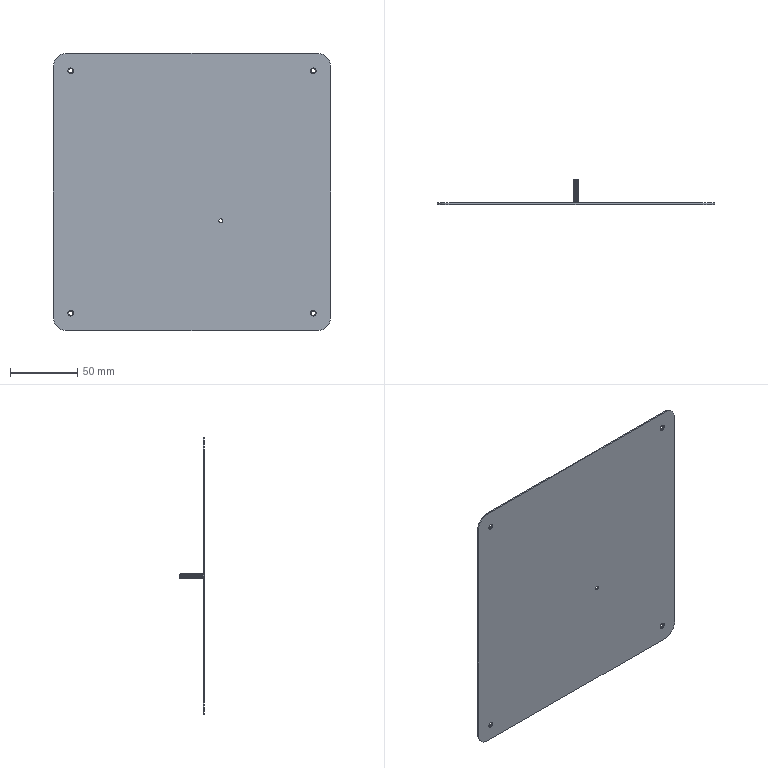Part | SolidWorks | features Chamfer 2, Extrusion 1, Helix 1, ICE 1, SweepCut 1 | 1 solid | 105 faces | box 206 x 18.5 x 206 mm | volume 42483 mm3 | cylinder 84 | cone 11 | plane 7 | spline 3 | commonest cylinder face diameters 3.8 x70 3.2 x8 20 x4 3 x2